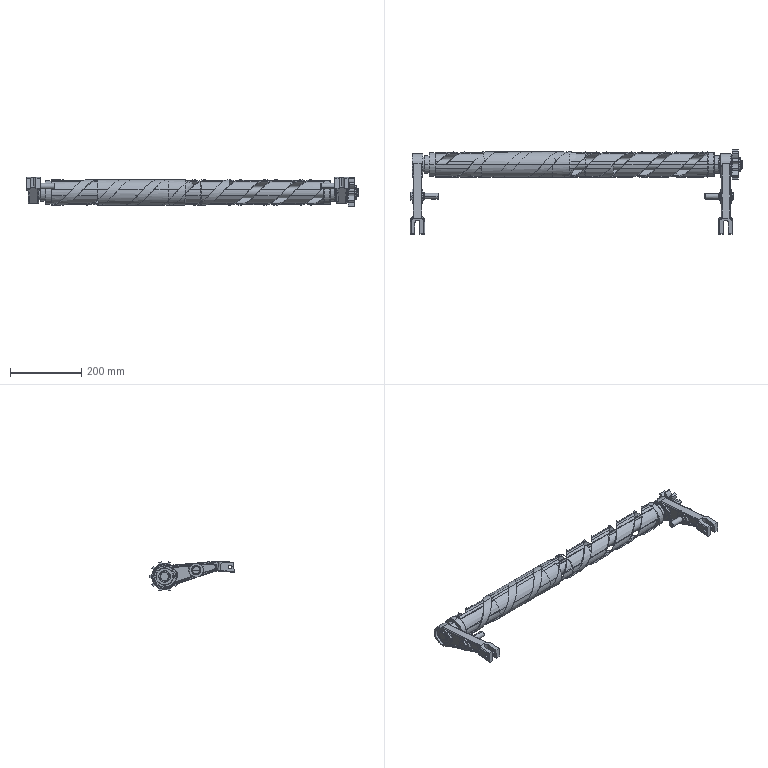Part | SolidWorks | features LayoutProfileFeature 1 | 15 solids | 865 faces | box 934.5 x 238.062 x 84.273 mm | volume 3595919 mm3 | cylinder 368 | spline 211 | plane 200 | cone 86 | commonest cylinder face diameters 4 x72 70 x42 65 x34 76.673 x22 25 x15 72 x14